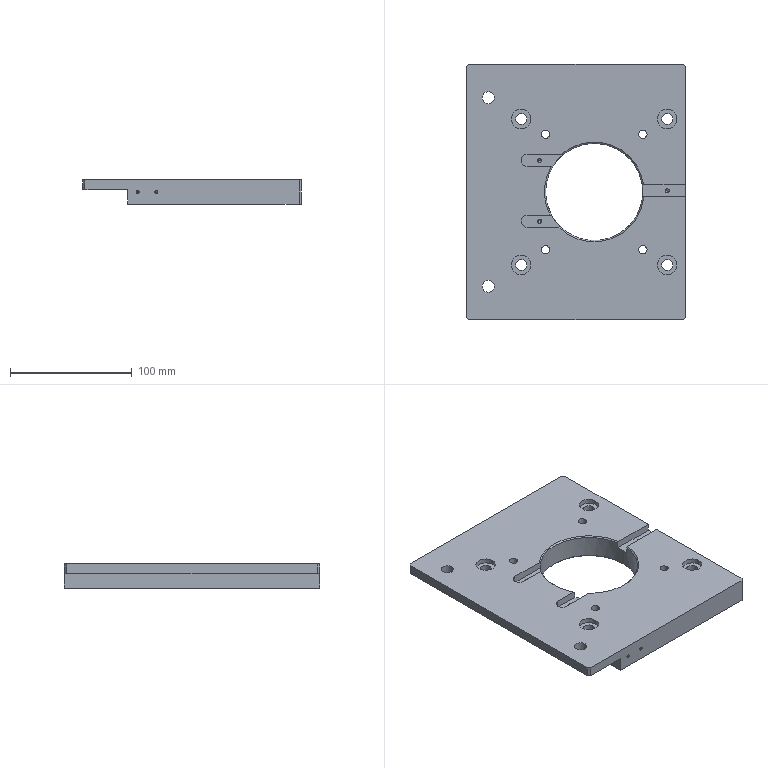Part | STEP file | PN_0012 Base | 1 solid | 144 faces | box 180 x 210 x 20 mm | volume 540025 mm3 | cylinder 76 | cone 39 | plane 29 | commonest cylinder face diameters 3.3 x22 2.5 x10 6.8 x8 9 x8 10 x8 14 x8